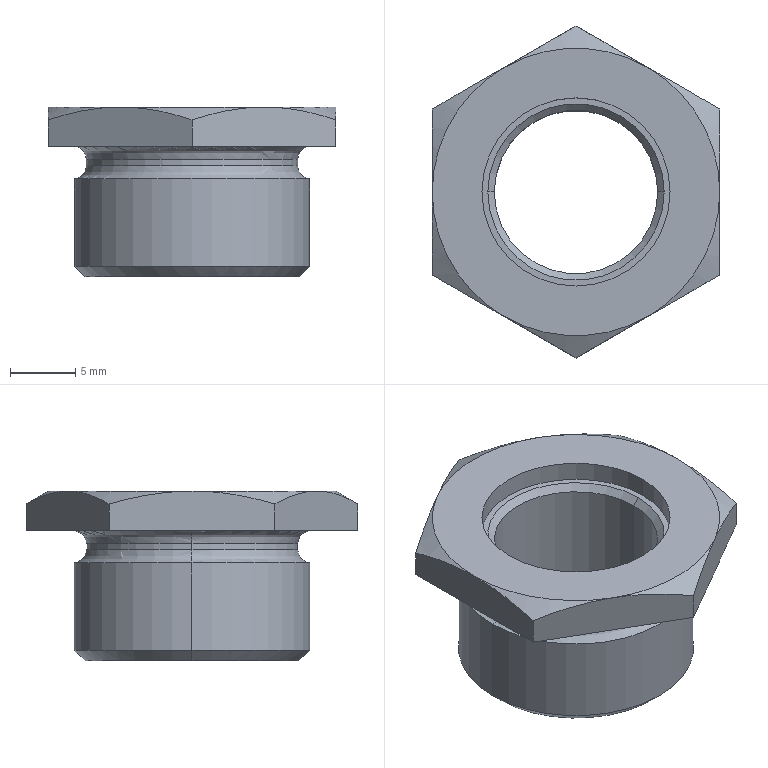Part | SolidWorks | features BaseBody 1 | 1 solid | 34 faces | box 22 x 25.403 x 13 mm | volume 2007 mm3 | cone 12 | plane 10 | cylinder 8 | torus 4 | commonest cylinder face diameters 12.5 x2 14.4 x2 16.2 x2 18 x2
STEP:
#1=CARTESIAN_POINT('',(49.25,110.5,49.));
#2=VERTEX_POINT('',#1);
#3=CARTESIAN_POINT('',(61.75,110.5,49.));
#4=VERTEX_POINT('',#3);
#5=CARTESIAN_POINT('',(55.5,110.5,49.));
#6=DIRECTION('',(0.,0.,1.));
#7=DIRECTION('',(1.,0.,0.));
#8=AXIS2_PLACEMENT_3D('',#5,#6,#7);
#9=CIRCLE('',#8,6.25);
#10=EDGE_CURVE('',#2,#4,#9,.T.);
#11=ORIENTED_EDGE('',*,*,#10,.F.);
#12=CARTESIAN_POINT('',(48.75,110.5,49.5));
#13=VERTEX_POINT('',#12);
#14=CARTESIAN_POINT('',(49.25,110.5,49.));
#15=DIRECTION('',(-0.7071,0.,0.7071));
#16=VECTOR('',#15,1000.);
#17=LINE('',#14,#16);
#18=EDGE_CURVE('',#2,#13,#17,.T.);
#19=ORIENTED_EDGE('',*,*,#18,.T.);
#20=CARTESIAN_POINT('',(62.25,110.5,49.5));
#21=VERTEX_POINT('',#20);
#22=CARTESIAN_POINT('',(55.5,110.5,49.5));
#23=DIRECTION('',(0.,0.,-1.));
#24=DIRECTION('',(1.,0.,0.));
#25=AXIS2_PLACEMENT_3D('',#22,#23,#24);
#26=CIRCLE('',#25,6.75);
#27=EDGE_CURVE('',#21,#13,#26,.T.);
#28=ORIENTED_EDGE('',*,*,#27,.F.);
#29=CARTESIAN_POINT('',(61.75,110.5,49.));
#30=DIRECTION('',(0.7071,0.,0.7071));
#31=VECTOR('',#30,1000.);
#32=LINE('',#29,#31);
#33=EDGE_CURVE('',#4,#21,#32,.T.);
#34=ORIENTED_EDGE('',*,*,#33,.F.);
#35=EDGE_LOOP('',(#11,#19,#28,#34));
#36=FACE_OUTER_BOUND('',#35,.T.);
#37=CARTESIAN_POINT('',(55.5,110.5,49.));
#38=DIRECTION('',(0.,0.,1.));
#39=DIRECTION('',(1.,0.,0.));
#40=AXIS2_PLACEMENT_3D('',#37,#38,#39);
#41=CONICAL_SURFACE('',#40,6.25,0.7854);
#42=ADVANCED_FACE('',(#36),#41,.F.);
#43=CARTESIAN_POINT('',(61.75,110.5,38.433));
#44=VERTEX_POINT('',#43);
#45=CARTESIAN_POINT('',(49.25,110.5,38.433));
#46=VERTEX_POINT('',#45);
#47=CARTESIAN_POINT('',(55.5,110.5,38.433));
#48=DIRECTION('',(0.,0.,-1.));
#49=DIRECTION('',(-1.,0.,0.));
#50=AXIS2_PLACEMENT_3D('',#47,#48,#49);
#51=CIRCLE('',#50,6.25);
#52=EDGE_CURVE('',#44,#46,#51,.T.);
#53=ORIENTED_EDGE('',*,*,#52,.F.);
#54=CARTESIAN_POINT('',(62.5,110.5,38.));
#55=VERTEX_POINT('',#54);
#56=CARTESIAN_POINT('',(62.5,110.5,38.));
#57=DIRECTION('',(0.866,0.,-0.5));
#58=VECTOR('',#57,1000.);
#59=LINE('',#56,#58);
#60=EDGE_CURVE('',#44,#55,#59,.T.);
#61=ORIENTED_EDGE('',*,*,#60,.T.);
#62=CARTESIAN_POINT('',(48.5,110.5,38.));
#63=VERTEX_POINT('',#62);
#64=CARTESIAN_POINT('',(55.5,110.5,38.));
#65=DIRECTION('',(0.,0.,-1.));
#66=DIRECTION('',(-1.,0.,0.));
#67=AXIS2_PLACEMENT_3D('',#64,#65,#66);
#68=CIRCLE('',#67,7.);
#69=EDGE_CURVE('',#55,#63,#68,.T.);
#70=ORIENTED_EDGE('',*,*,#69,.T.);
#71=CARTESIAN_POINT('',(48.5,110.5,38.));
#72=DIRECTION('',(-0.866,0.,-0.5));
#73=VECTOR('',#72,1000.);
#74=LINE('',#71,#73);
#75=EDGE_CURVE('',#46,#63,#74,.T.);
#76=ORIENTED_EDGE('',*,*,#75,.F.);
#77=EDGE_LOOP('',(#53,#61,#70,#76));
#78=FACE_OUTER_BOUND('',#77,.T.);
#79=CARTESIAN_POINT('',(55.5,110.5,38.));
#80=DIRECTION('',(0.,0.,-1.));
#81=DIRECTION('',(-1.,0.,0.));
#82=AXIS2_PLACEMENT_3D('',#79,#80,#81);
#83=CONICAL_SURFACE('',#82,7.,1.047);
#84=ADVANCED_FACE('',(#78),#83,.F.);
#85=ORIENTED_EDGE('',*,*,#10,.T.);
#86=CARTESIAN_POINT('',(61.75,110.5,38.));
#87=DIRECTION('',(0.,0.,-1.));
#88=VECTOR('',#87,1000.);
#89=LINE('',#86,#88);
#90=EDGE_CURVE('',#4,#44,#89,.T.);
#91=ORIENTED_EDGE('',*,*,#90,.T.);
#92=ORIENTED_EDGE('',*,*,#52,.T.);
#93=CARTESIAN_POINT('',(49.25,110.5,38.));
#94=DIRECTION('',(0.,0.,-1.));
#95=VECTOR('',#94,1000.);
#96=LINE('',#93,#95);
#97=EDGE_CURVE('',#2,#46,#96,.T.);
#98=ORIENTED_EDGE('',*,*,#97,.F.);
#99=EDGE_LOOP('',(#85,#91,#92,#98));
#100=FACE_OUTER_BOUND('',#99,.T.);
#101=CARTESIAN_POINT('',(55.5,110.5,38.));
#102=DIRECTION('',(0.,0.,-1.));
#103=DIRECTION('',(-1.,0.,0.));
#104=AXIS2_PLACEMENT_3D('',#101,#102,#103);
#105=CYLINDRICAL_SURFACE('',#104,6.25);
#106=ADVANCED_FACE('',(#100),#105,.F.);
#107=CARTESIAN_POINT('',(48.3,110.5,49.5));
#108=VERTEX_POINT('',#107);
#109=CARTESIAN_POINT('',(62.7,110.5,49.5));
#110=VERTEX_POINT('',#109);
#111=CARTESIAN_POINT('',(55.5,110.5,49.5));
#112=DIRECTION('',(0.,0.,1.));
#113=DIRECTION('',(1.,0.,0.));
#114=AXIS2_PLACEMENT_3D('',#111,#112,#113);
#115=CIRCLE('',#114,7.2);
#116=EDGE_CURVE('',#108,#110,#115,.T.);
#117=ORIENTED_EDGE('',*,*,#116,.F.);
#118=CARTESIAN_POINT('',(48.3,110.5,51.));
#119=VERTEX_POINT('',#118);
#120=CARTESIAN_POINT('',(48.3,110.5,49.5));
#121=DIRECTION('',(0.,0.,1.));
#122=VECTOR('',#121,1000.);
#123=LINE('',#120,#122);
#124=EDGE_CURVE('',#108,#119,#123,.T.);
#125=ORIENTED_EDGE('',*,*,#124,.T.);
#126=CARTESIAN_POINT('',(62.7,110.5,51.));
#127=VERTEX_POINT('',#126);
#128=CARTESIAN_POINT('',(55.5,110.5,51.));
#129=DIRECTION('',(0.,0.,1.));
#130=DIRECTION('',(1.,0.,0.));
#131=AXIS2_PLACEMENT_3D('',#128,#129,#130);
#132=CIRCLE('',#131,7.2);
#133=EDGE_CURVE('',#119,#127,#132,.T.);
#134=ORIENTED_EDGE('',*,*,#133,.T.);
#135=CARTESIAN_POINT('',(62.7,110.5,49.5));
#136=DIRECTION('',(0.,0.,1.));
#137=VECTOR('',#136,1000.);
#138=LINE('',#135,#137);
#139=EDGE_CURVE('',#110,#127,#138,.T.);
#140=ORIENTED_EDGE('',*,*,#139,.F.);
#141=EDGE_LOOP('',(#117,#125,#134,#140));
#142=FACE_OUTER_BOUND('',#141,.T.);
#143=CARTESIAN_POINT('',(55.5,110.5,49.5));
#144=DIRECTION('',(0.,0.,1.));
#145=DIRECTION('',(1.,0.,0.));
#146=AXIS2_PLACEMENT_3D('',#143,#144,#145);
#147=CYLINDRICAL_SURFACE('',#146,7.2);
#148=ADVANCED_FACE('',(#142),#147,.F.);
#149=CARTESIAN_POINT('',(63.6,110.5,47.005));
#150=VERTEX_POINT('',#149);
#151=CARTESIAN_POINT('',(47.4,110.5,47.005));
#152=VERTEX_POINT('',#151);
#153=CARTESIAN_POINT('',(55.5,110.5,47.005));
#154=DIRECTION('',(0.,0.,-1.));
#155=DIRECTION('',(-1.,0.,0.));
#156=AXIS2_PLACEMENT_3D('',#153,#154,#155);
#157=CIRCLE('',#156,8.1);
#158=EDGE_CURVE('',#150,#152,#157,.T.);
#159=ORIENTED_EDGE('',*,*,#158,.F.);
#160=CARTESIAN_POINT('',(64.5,110.5,48.));
#161=VERTEX_POINT('',#160);
#162=CARTESIAN_POINT('',(64.6,110.5,47.005));
#163=DIRECTION('',(0.,1.,0.));
#164=DIRECTION('',(-1.,0.,0.));
#165=AXIS2_PLACEMENT_3D('',#162,#163,#164);
#166=CIRCLE('',#165,1.);
#167=EDGE_CURVE('',#150,#161,#166,.T.);
#168=ORIENTED_EDGE('',*,*,#167,.T.);
#169=CARTESIAN_POINT('',(46.5,110.5,48.));
#170=VERTEX_POINT('',#169);
#171=CARTESIAN_POINT('',(55.5,110.5,48.));
#172=DIRECTION('',(0.,0.,1.));
#173=DIRECTION('',(1.,0.,0.));
#174=AXIS2_PLACEMENT_3D('',#171,#172,#173);
#175=CIRCLE('',#174,9.);
#176=EDGE_CURVE('',#170,#161,#175,.T.);
#177=ORIENTED_EDGE('',*,*,#176,.F.);
#178=CARTESIAN_POINT('',(46.4,110.5,47.005));
#179=DIRECTION('',(0.,-1.,0.));
#180=DIRECTION('',(1.,0.,0.));
#181=AXIS2_PLACEMENT_3D('',#178,#179,#180);
#182=CIRCLE('',#181,1.);
#183=EDGE_CURVE('',#152,#170,#182,.T.);
#184=ORIENTED_EDGE('',*,*,#183,.F.);
#185=EDGE_LOOP('',(#159,#168,#177,#184));
#186=FACE_OUTER_BOUND('',#185,.T.);
#187=CARTESIAN_POINT('',(55.5,110.5,47.005));
#188=DIRECTION('',(0.,0.,-1.));
#189=DIRECTION('',(-1.,0.,0.));
#190=AXIS2_PLACEMENT_3D('',#187,#188,#189);
#191=TOROIDAL_SURFACE('',#190,9.1,1.);
#192=ADVANCED_FACE('',(#186),#191,.F.);
#193=CARTESIAN_POINT('',(55.5,110.5,47.005));
#194=DIRECTION('',(0.,0.,-1.));
#195=DIRECTION('',(-1.,0.,0.));
#196=AXIS2_PLACEMENT_3D('',#193,#194,#195);
#197=CIRCLE('',#196,8.1);
#198=EDGE_CURVE('',#152,#150,#197,.T.);
#199=ORIENTED_EDGE('',*,*,#198,.T.);
#200=CARTESIAN_POINT('',(63.6,110.5,46.495));
#201=VERTEX_POINT('',#200);
#202=CARTESIAN_POINT('',(63.6,110.5,38.));
#203=DIRECTION('',(0.,0.,-1.));
#204=VECTOR('',#203,1000.);
#205=LINE('',#202,#204);
#206=EDGE_CURVE('',#150,#201,#205,.T.);
#207=ORIENTED_EDGE('',*,*,#206,.T.);
#208=CARTESIAN_POINT('',(47.4,110.5,46.495));
#209=VERTEX_POINT('',#208);
#210=CARTESIAN_POINT('',(55.5,110.5,46.495));
#211=DIRECTION('',(0.,0.,-1.));
#212=DIRECTION('',(-1.,0.,0.));
#213=AXIS2_PLACEMENT_3D('',#210,#211,#212);
#214=CIRCLE('',#213,8.1);
#215=EDGE_CURVE('',#209,#201,#214,.T.);
#216=ORIENTED_EDGE('',*,*,#215,.F.);
#217=CARTESIAN_POINT('',(47.4,110.5,38.));
#218=DIRECTION('',(0.,0.,-1.));
#219=VECTOR('',#218,1000.);
#220=LINE('',#217,#219);
#221=EDGE_CURVE('',#152,#209,#220,.T.);
#222=ORIENTED_EDGE('',*,*,#221,.F.);
#223=EDGE_LOOP('',(#199,#207,#216,#222));
#224=FACE_OUTER_BOUND('',#223,.T.);
#225=CARTESIAN_POINT('',(55.5,110.5,38.));
#226=DIRECTION('',(0.,0.,-1.));
#227=DIRECTION('',(-1.,0.,0.));
#228=AXIS2_PLACEMENT_3D('',#225,#226,#227);
#229=CYLINDRICAL_SURFACE('',#228,8.1);
#230=ADVANCED_FACE('',(#224),#229,.T.);
#231=CARTESIAN_POINT('',(64.5,110.5,45.5));
#232=VERTEX_POINT('',#231);
#233=CARTESIAN_POINT('',(46.5,110.5,45.5));
#234=VERTEX_POINT('',#233);
#235=CARTESIAN_POINT('',(55.5,110.5,45.5));
#236=DIRECTION('',(0.,0.,-1.));
#237=DIRECTION('',(-1.,0.,0.));
#238=AXIS2_PLACEMENT_3D('',#235,#236,#237);
#239=CIRCLE('',#238,9.);
#240=EDGE_CURVE('',#232,#234,#239,.T.);
#241=ORIENTED_EDGE('',*,*,#240,.F.);
#242=CARTESIAN_POINT('',(64.6,110.5,46.495));
#243=DIRECTION('',(0.,1.,0.));
#244=DIRECTION('',(-1.,0.,0.));
#245=AXIS2_PLACEMENT_3D('',#242,#243,#244);
#246=CIRCLE('',#245,1.);
#247=EDGE_CURVE('',#232,#201,#246,.T.);
#248=ORIENTED_EDGE('',*,*,#247,.T.);
#249=CARTESIAN_POINT('',(55.5,110.5,46.495));
#250=DIRECTION('',(0.,0.,-1.));
#251=DIRECTION('',(-1.,0.,0.));
#252=AXIS2_PLACEMENT_3D('',#249,#250,#251);
#253=CIRCLE('',#252,8.1);
#254=EDGE_CURVE('',#201,#209,#253,.T.);
#255=ORIENTED_EDGE('',*,*,#254,.T.);
#256=CARTESIAN_POINT('',(46.4,110.5,46.495));
#257=DIRECTION('',(0.,-1.,0.));
#258=DIRECTION('',(1.,0.,0.));
#259=AXIS2_PLACEMENT_3D('',#256,#257,#258);
#260=CIRCLE('',#259,1.);
#261=EDGE_CURVE('',#234,#209,#260,.T.);
#262=ORIENTED_EDGE('',*,*,#261,.F.);
#263=EDGE_LOOP('',(#241,#248,#255,#262));
#264=FACE_OUTER_BOUND('',#263,.T.);
#265=CARTESIAN_POINT('',(55.5,110.5,46.495));
#266=DIRECTION('',(0.,0.,-1.));
#267=DIRECTION('',(-1.,0.,0.));
#268=AXIS2_PLACEMENT_3D('',#265,#266,#267);
#269=TOROIDAL_SURFACE('',#268,9.1,1.);
#270=ADVANCED_FACE('',(#264),#269,.F.);
#271=CARTESIAN_POINT('',(55.5,110.5,45.5));
#272=DIRECTION('',(0.,0.,-1.));
#273=DIRECTION('',(-1.,0.,0.));
#274=AXIS2_PLACEMENT_3D('',#271,#272,#273);
#275=CIRCLE('',#274,9.);
#276=EDGE_CURVE('',#234,#232,#275,.T.);
#277=ORIENTED_EDGE('',*,*,#276,.T.);
#278=CARTESIAN_POINT('',(64.5,110.5,38.8));
#279=VERTEX_POINT('',#278);
#280=CARTESIAN_POINT('',(64.5,110.5,38.));
#281=DIRECTION('',(0.,0.,-1.));
#282=VECTOR('',#281,1000.);
#283=LINE('',#280,#282);
#284=EDGE_CURVE('',#232,#279,#283,.T.);
#285=ORIENTED_EDGE('',*,*,#284,.T.);
#286=CARTESIAN_POINT('',(46.5,110.5,38.8));
#287=VERTEX_POINT('',#286);
#288=CARTESIAN_POINT('',(55.5,110.5,38.8));
#289=DIRECTION('',(0.,0.,-1.));
#290=DIRECTION('',(-1.,0.,0.));
#291=AXIS2_PLACEMENT_3D('',#288,#289,#290);
#292=CIRCLE('',#291,9.);
#293=EDGE_CURVE('',#287,#279,#292,.T.);
#294=ORIENTED_EDGE('',*,*,#293,.F.);
#295=CARTESIAN_POINT('',(46.5,110.5,38.));
#296=DIRECTION('',(0.,0.,-1.));
#297=VECTOR('',#296,1000.);
#298=LINE('',#295,#297);
#299=EDGE_CURVE('',#234,#287,#298,.T.);
#300=ORIENTED_EDGE('',*,*,#299,.F.);
#301=EDGE_LOOP('',(#277,#285,#294,#300));
#302=FACE_OUTER_BOUND('',#301,.T.);
#303=CARTESIAN_POINT('',(55.5,110.5,38.));
#304=DIRECTION('',(0.,0.,-1.));
#305=DIRECTION('',(-1.,0.,0.));
#306=AXIS2_PLACEMENT_3D('',#303,#304,#305);
#307=CYLINDRICAL_SURFACE('',#306,9.);
#308=ADVANCED_FACE('',(#302),#307,.T.);
#309=CARTESIAN_POINT('',(47.3,110.5,38.));
#310=VERTEX_POINT('',#309);
#311=CARTESIAN_POINT('',(63.7,110.5,38.));
#312=VERTEX_POINT('',#311);
#313=CARTESIAN_POINT('',(55.5,110.5,38.));
#314=DIRECTION('',(0.,0.,-1.));
#315=DIRECTION('',(-1.,0.,0.));
#316=AXIS2_PLACEMENT_3D('',#313,#314,#315);
#317=CIRCLE('',#316,8.2);
#318=EDGE_CURVE('',#310,#312,#317,.T.);
#319=ORIENTED_EDGE('',*,*,#318,.F.);
#320=CARTESIAN_POINT('',(47.3,110.5,38.));
#321=DIRECTION('',(-0.7071,0.,0.7071));
#322=VECTOR('',#321,1000.);
#323=LINE('',#320,#322);
#324=EDGE_CURVE('',#310,#287,#323,.T.);
#325=ORIENTED_EDGE('',*,*,#324,.T.);
#326=ORIENTED_EDGE('',*,*,#293,.T.);
#327=CARTESIAN_POINT('',(63.7,110.5,38.));
#328=DIRECTION('',(0.7071,0.,0.7071));
#329=VECTOR('',#328,1000.);
#330=LINE('',#327,#329);
#331=EDGE_CURVE('',#312,#279,#330,.T.);
#332=ORIENTED_EDGE('',*,*,#331,.F.);
#333=EDGE_LOOP('',(#319,#325,#326,#332));
#334=FACE_OUTER_BOUND('',#333,.T.);
#335=CARTESIAN_POINT('',(55.5,110.5,38.));
#336=DIRECTION('',(0.,0.,1.));
#337=DIRECTION('',(1.,0.,0.));
#338=AXIS2_PLACEMENT_3D('',#335,#336,#337);
#339=CONICAL_SURFACE('',#338,8.2,0.7854);
#340=ADVANCED_FACE('',(#334),#339,.T.);
#341=CARTESIAN_POINT('',(44.5,104.149,50.018));
#342=VERTEX_POINT('',#341);
#343=CARTESIAN_POINT('',(50.,100.974,51.));
#344=VERTEX_POINT('',#343);
#345=CARTESIAN_POINT('',(44.5,104.149,50.018));
#346=CARTESIAN_POINT('',(45.4,103.63,50.317));
#347=CARTESIAN_POINT('',(46.306,103.106,50.565));
#348=CARTESIAN_POINT('',(48.138,102.049,50.906));
#349=CARTESIAN_POINT('',(49.063,101.515,51.));
#350=CARTESIAN_POINT('',(50.,100.974,51.));
#351=B_SPLINE_CURVE_WITH_KNOTS('',3,(#345,#346,#347,#348,#349,#350),.UNSPECIFIED.,.F.,.F.,(4,2,4),(0.000000238,0.003213,0.006426),.UNSPECIFIED.);
#352=EDGE_CURVE('',#342,#344,#351,.T.);
#353=ORIENTED_EDGE('',*,*,#352,.F.);
#354=CARTESIAN_POINT('',(44.5,104.149,48.));
#355=VERTEX_POINT('',#354);
#356=CARTESIAN_POINT('',(44.5,104.149,97.606));
#357=DIRECTION('',(0.,0.,-1.));
#358=VECTOR('',#357,1000.);
#359=LINE('',#356,#358);
#360=EDGE_CURVE('',#342,#355,#359,.T.);
#361=ORIENTED_EDGE('',*,*,#360,.T.);
#362=CARTESIAN_POINT('',(55.5,97.798,48.));
#363=VERTEX_POINT('',#362);
#364=CARTESIAN_POINT('',(44.5,104.149,48.));
#365=DIRECTION('',(0.866,-0.5,0.));
#366=VECTOR('',#365,1000.);
#367=LINE('',#364,#366);
#368=EDGE_CURVE('',#355,#363,#367,.T.);
#369=ORIENTED_EDGE('',*,*,#368,.T.);
#370=CARTESIAN_POINT('',(55.5,97.798,50.018));
#371=VERTEX_POINT('',#370);
#372=CARTESIAN_POINT('',(55.5,97.798,97.606));
#373=DIRECTION('',(0.,0.,-1.));
#374=VECTOR('',#373,1000.);
#375=LINE('',#372,#374);
#376=EDGE_CURVE('',#371,#363,#375,.T.);
#377=ORIENTED_EDGE('',*,*,#376,.F.);
#378=CARTESIAN_POINT('',(50.,100.974,51.));
#379=CARTESIAN_POINT('',(50.467,100.704,51.));
#380=CARTESIAN_POINT('',(50.936,100.434,50.977));
#381=CARTESIAN_POINT('',(51.863,99.898,50.887));
#382=CARTESIAN_POINT('',(52.324,99.632,50.82));
#383=CARTESIAN_POINT('',(53.698,98.839,50.564));
#384=CARTESIAN_POINT('',(54.603,98.316,50.317));
#385=CARTESIAN_POINT('',(55.5,97.798,50.018));
#386=B_SPLINE_CURVE_WITH_KNOTS('',3,(#378,#379,#380,#381,#382,#383,#384,#385),.UNSPECIFIED.,.F.,.F.,(4,2,2,4),(0.006426,0.008027,0.009627,0.01283),.UNSPECIFIED.);
#387=EDGE_CURVE('',#344,#371,#386,.T.);
#388=ORIENTED_EDGE('',*,*,#387,.F.);
#389=EDGE_LOOP('',(#353,#361,#369,#377,#388));
#390=FACE_OUTER_BOUND('',#389,.T.);
#391=CARTESIAN_POINT('',(44.5,104.149,97.606));
#392=DIRECTION('',(0.5,0.866,0.));
#393=DIRECTION('',(-0.866,0.5,0.));
#394=AXIS2_PLACEMENT_3D('',#391,#392,#393);
#395=PLANE('',#394);
#396=ADVANCED_FACE('',(#390),#395,.F.);
#397=CARTESIAN_POINT('',(44.5,116.851,50.018));
#398=VERTEX_POINT('',#397);
#399=CARTESIAN_POINT('',(44.5,110.5,51.));
#400=VERTEX_POINT('',#399);
#401=CARTESIAN_POINT('',(44.5,116.851,50.018));
#402=CARTESIAN_POINT('',(44.5,115.824,50.314));
#403=CARTESIAN_POINT('',(44.5,114.784,50.561));
#404=CARTESIAN_POINT('',(44.5,113.194,50.819));
#405=CARTESIAN_POINT('',(44.5,112.659,50.886));
#406=CARTESIAN_POINT('',(44.5,111.577,50.977));
#407=CARTESIAN_POINT('',(44.5,111.037,51.));
#408=CARTESIAN_POINT('',(44.5,110.5,51.));
#409=B_SPLINE_CURVE_WITH_KNOTS('',3,(#401,#402,#403,#404,#405,#406,#407,#408),.UNSPECIFIED.,.F.,.F.,(4,2,2,4),(0.02901,0.03222,0.03383,0.03544),.UNSPECIFIED.);
#410=EDGE_CURVE('',#398,#400,#409,.T.);
#411=ORIENTED_EDGE('',*,*,#410,.F.);
#412=CARTESIAN_POINT('',(44.5,116.851,48.));
#413=VERTEX_POINT('',#412);
#414=CARTESIAN_POINT('',(44.5,116.851,97.606));
#415=DIRECTION('',(0.,0.,-1.));
#416=VECTOR('',#415,1000.);
#417=LINE('',#414,#416);
#418=EDGE_CURVE('',#398,#413,#417,.T.);
#419=ORIENTED_EDGE('',*,*,#418,.T.);
#420=CARTESIAN_POINT('',(44.5,116.851,48.));
#421=DIRECTION('',(0.,-1.,0.));
#422=VECTOR('',#421,1000.);
#423=LINE('',#420,#422);
#424=EDGE_CURVE('',#413,#355,#423,.T.);
#425=ORIENTED_EDGE('',*,*,#424,.T.);
#426=ORIENTED_EDGE('',*,*,#360,.F.);
#427=CARTESIAN_POINT('',(44.5,110.5,51.));
#428=CARTESIAN_POINT('',(44.5,109.426,51.));
#429=CARTESIAN_POINT('',(44.5,108.36,50.908));
#430=CARTESIAN_POINT('',(44.5,106.24,50.566));
#431=CARTESIAN_POINT('',(44.5,105.183,50.316));
#432=CARTESIAN_POINT('',(44.5,104.149,50.018));
#433=B_SPLINE_CURVE_WITH_KNOTS('',3,(#427,#428,#429,#430,#431,#432),.UNSPECIFIED.,.F.,.F.,(4,2,4),(0.03544,0.03866,0.04187),.UNSPECIFIED.);
#434=EDGE_CURVE('',#400,#342,#433,.T.);
#435=ORIENTED_EDGE('',*,*,#434,.F.);
#436=EDGE_LOOP('',(#411,#419,#425,#426,#435));
#437=FACE_OUTER_BOUND('',#436,.T.);
#438=CARTESIAN_POINT('',(44.5,116.851,97.606));
#439=DIRECTION('',(1.,0.,0.));
#440=DIRECTION('',(0.,1.,0.));
#441=AXIS2_PLACEMENT_3D('',#438,#439,#440);
#442=PLANE('',#441);
#443=ADVANCED_FACE('',(#437),#442,.F.);
#444=CARTESIAN_POINT('',(55.5,123.202,50.018));
#445=VERTEX_POINT('',#444);
#446=CARTESIAN_POINT('',(50.,120.026,51.));
#447=VERTEX_POINT('',#446);
#448=CARTESIAN_POINT('',(55.5,123.202,50.018));
#449=CARTESIAN_POINT('',(54.6,122.682,50.317));
#450=CARTESIAN_POINT('',(53.694,122.159,50.565));
#451=CARTESIAN_POINT('',(51.862,121.102,50.906));
#452=CARTESIAN_POINT('',(50.937,120.567,51.));
#453=CARTESIAN_POINT('',(50.,120.026,51.));
#454=B_SPLINE_CURVE_WITH_KNOTS('',3,(#448,#449,#450,#451,#452,#453),.UNSPECIFIED.,.F.,.F.,(4,2,4),(0.000000238,0.003213,0.006426),.UNSPECIFIED.);
#455=EDGE_CURVE('',#445,#447,#454,.T.);
#456=ORIENTED_EDGE('',*,*,#455,.F.);
#457=CARTESIAN_POINT('',(55.5,123.202,48.));
#458=VERTEX_POINT('',#457);
#459=CARTESIAN_POINT('',(55.5,123.202,97.606));
#460=DIRECTION('',(0.,0.,-1.));
#461=VECTOR('',#460,1000.);
#462=LINE('',#459,#461);
#463=EDGE_CURVE('',#445,#458,#462,.T.);
#464=ORIENTED_EDGE('',*,*,#463,.T.);
#465=CARTESIAN_POINT('',(55.5,123.202,48.));
#466=DIRECTION('',(-0.866,-0.5,0.));
#467=VECTOR('',#466,1000.);
#468=LINE('',#465,#467);
#469=EDGE_CURVE('',#458,#413,#468,.T.);
#470=ORIENTED_EDGE('',*,*,#469,.T.);
#471=ORIENTED_EDGE('',*,*,#418,.F.);
#472=CARTESIAN_POINT('',(50.,120.026,51.));
#473=CARTESIAN_POINT('',(49.533,119.757,51.));
#474=CARTESIAN_POINT('',(49.064,119.486,50.977));
#475=CARTESIAN_POINT('',(48.137,118.951,50.887));
#476=CARTESIAN_POINT('',(47.676,118.685,50.82));
#477=CARTESIAN_POINT('',(46.302,117.891,50.564));
#478=CARTESIAN_POINT('',(45.397,117.369,50.317));
#479=CARTESIAN_POINT('',(44.5,116.851,50.018));
#480=B_SPLINE_CURVE_WITH_KNOTS('',3,(#472,#473,#474,#475,#476,#477,#478,#479),.UNSPECIFIED.,.F.,.F.,(4,2,2,4),(0.006426,0.008027,0.009627,0.01283),.UNSPECIFIED.);
#481=EDGE_CURVE('',#447,#398,#480,.T.);
#482=ORIENTED_EDGE('',*,*,#481,.F.);
#483=EDGE_LOOP('',(#456,#464,#470,#471,#482));
#484=FACE_OUTER_BOUND('',#483,.T.);
#485=CARTESIAN_POINT('',(55.5,123.202,97.606));
#486=DIRECTION('',(0.5,-0.866,0.));
#487=DIRECTION('',(0.866,0.5,0.));
#488=AXIS2_PLACEMENT_3D('',#485,#486,#487);
#489=PLANE('',#488);
#490=ADVANCED_FACE('',(#484),#489,.F.);
#491=CARTESIAN_POINT('',(66.5,116.851,50.018));
#492=VERTEX_POINT('',#491);
#493=CARTESIAN_POINT('',(61.,120.026,51.));
#494=VERTEX_POINT('',#493);
#495=CARTESIAN_POINT('',(66.5,116.851,50.018));
#496=CARTESIAN_POINT('',(65.6,117.37,50.317));
#497=CARTESIAN_POINT('',(64.694,117.894,50.565));
#498=CARTESIAN_POINT('',(62.862,118.951,50.906));
#499=CARTESIAN_POINT('',(61.937,119.485,51.));
#500=CARTESIAN_POINT('',(61.,120.026,51.));
#501=B_SPLINE_CURVE_WITH_KNOTS('',3,(#495,#496,#497,#498,#499,#500),.UNSPECIFIED.,.F.,.F.,(4,2,4),(0.000000238,0.003213,0.006426),.UNSPECIFIED.);
#502=EDGE_CURVE('',#492,#494,#501,.T.);
#503=ORIENTED_EDGE('',*,*,#502,.F.);
#504=CARTESIAN_POINT('',(66.5,116.851,48.));
#505=VERTEX_POINT('',#504);
#506=CARTESIAN_POINT('',(66.5,116.851,97.606));
#507=DIRECTION('',(0.,0.,-1.));
#508=VECTOR('',#507,1000.);
#509=LINE('',#506,#508);
#510=EDGE_CURVE('',#492,#505,#509,.T.);
#511=ORIENTED_EDGE('',*,*,#510,.T.);
#512=CARTESIAN_POINT('',(66.5,116.851,48.));
#513=DIRECTION('',(-0.866,0.5,0.));
#514=VECTOR('',#513,1000.);
#515=LINE('',#512,#514);
#516=EDGE_CURVE('',#505,#458,#515,.T.);
#517=ORIENTED_EDGE('',*,*,#516,.T.);
#518=ORIENTED_EDGE('',*,*,#463,.F.);
#519=CARTESIAN_POINT('',(61.,120.026,51.));
#520=CARTESIAN_POINT('',(60.533,120.296,51.));
#521=CARTESIAN_POINT('',(60.064,120.566,50.977));
#522=CARTESIAN_POINT('',(59.137,121.102,50.887));
#523=CARTESIAN_POINT('',(58.676,121.368,50.82));
#524=CARTESIAN_POINT('',(57.302,122.161,50.564));
#525=CARTESIAN_POINT('',(56.397,122.684,50.317));
#526=CARTESIAN_POINT('',(55.5,123.202,50.018));
#527=B_SPLINE_CURVE_WITH_KNOTS('',3,(#519,#520,#521,#522,#523,#524,#525,#526),.UNSPECIFIED.,.F.,.F.,(4,2,2,4),(0.006426,0.008027,0.009627,0.01283),.UNSPECIFIED.);
#528=EDGE_CURVE('',#494,#445,#527,.T.);
#529=ORIENTED_EDGE('',*,*,#528,.F.);
#530=EDGE_LOOP('',(#503,#511,#517,#518,#529));
#531=FACE_OUTER_BOUND('',#530,.T.);
#532=CARTESIAN_POINT('',(66.5,116.851,97.606));
#533=DIRECTION('',(-0.5,-0.866,0.));
#534=DIRECTION('',(0.866,-0.5,0.));
#535=AXIS2_PLACEMENT_3D('',#532,#533,#534);
#536=PLANE('',#535);
#537=ADVANCED_FACE('',(#531),#536,.F.);
#538=CARTESIAN_POINT('',(66.5,104.149,50.018));
#539=VERTEX_POINT('',#538);
#540=CARTESIAN_POINT('',(66.5,110.5,51.));
#541=VERTEX_POINT('',#540);
#542=CARTESIAN_POINT('',(66.5,104.149,50.018));
#543=CARTESIAN_POINT('',(66.5,105.183,50.316));
#544=CARTESIAN_POINT('',(66.5,106.24,50.566));
#545=CARTESIAN_POINT('',(66.5,108.36,50.908));
#546=CARTESIAN_POINT('',(66.5,109.426,51.));
#547=CARTESIAN_POINT('',(66.5,110.5,51.));
#548=B_SPLINE_CURVE_WITH_KNOTS('',3,(#542,#543,#544,#545,#546,#547),.UNSPECIFIED.,.F.,.F.,(4,2,4),(0.01164,0.01486,0.01807),.UNSPECIFIED.);
#549=EDGE_CURVE('',#539,#541,#548,.T.);
#550=ORIENTED_EDGE('',*,*,#549,.F.);
#551=CARTESIAN_POINT('',(66.5,104.149,48.));
#552=VERTEX_POINT('',#551);
#553=CARTESIAN_POINT('',(66.5,104.149,97.606));
#554=DIRECTION('',(0.,0.,-1.));
#555=VECTOR('',#554,1000.);
#556=LINE('',#553,#555);
#557=EDGE_CURVE('',#539,#552,#556,.T.);
#558=ORIENTED_EDGE('',*,*,#557,.T.);
#559=CARTESIAN_POINT('',(66.5,104.149,48.));
#560=DIRECTION('',(0.,1.,0.));
#561=VECTOR('',#560,1000.);
#562=LINE('',#559,#561);
#563=EDGE_CURVE('',#552,#505,#562,.T.);
#564=ORIENTED_EDGE('',*,*,#563,.T.);
#565=ORIENTED_EDGE('',*,*,#510,.F.);
#566=CARTESIAN_POINT('',(66.5,110.5,51.));
#567=CARTESIAN_POINT('',(66.5,111.037,51.));
#568=CARTESIAN_POINT('',(66.5,111.577,50.977));
#569=CARTESIAN_POINT('',(66.5,112.659,50.886));
#570=CARTESIAN_POINT('',(66.5,113.194,50.819));
#571=CARTESIAN_POINT('',(66.5,114.784,50.561));
#572=CARTESIAN_POINT('',(66.5,115.824,50.314));
#573=CARTESIAN_POINT('',(66.5,116.851,50.018));
#574=B_SPLINE_CURVE_WITH_KNOTS('',3,(#566,#567,#568,#569,#570,#571,#572,#573),.UNSPECIFIED.,.F.,.F.,(4,2,2,4),(0.01807,0.01968,0.02129,0.0245),.UNSPECIFIED.);
#575=EDGE_CURVE('',#541,#492,#574,.T.);
#576=ORIENTED_EDGE('',*,*,#575,.F.);
#577=EDGE_LOOP('',(#550,#558,#564,#565,#576));
#578=FACE_OUTER_BOUND('',#577,.T.);
#579=CARTESIAN_POINT('',(66.5,104.149,97.606));
#580=DIRECTION('',(-1.,0.,0.));
#581=DIRECTION('',(0.,-1.,0.));
#582=AXIS2_PLACEMENT_3D('',#579,#580,#581);
#583=PLANE('',#582);
#584=ADVANCED_FACE('',(#578),#583,.F.);
#585=CARTESIAN_POINT('',(61.,100.974,51.));
#586=VERTEX_POINT('',#585);
#587=CARTESIAN_POINT('',(55.5,97.798,50.018));
#588=CARTESIAN_POINT('',(56.4,98.318,50.317));
#589=CARTESIAN_POINT('',(57.306,98.841,50.565));
#590=CARTESIAN_POINT('',(59.138,99.898,50.906));
#591=CARTESIAN_POINT('',(60.063,100.433,51.));
#592=CARTESIAN_POINT('',(61.,100.974,51.));
#593=B_SPLINE_CURVE_WITH_KNOTS('',3,(#587,#588,#589,#590,#591,#592),.UNSPECIFIED.,.F.,.F.,(4,2,4),(0.000000238,0.003213,0.006426),.UNSPECIFIED.);
#594=EDGE_CURVE('',#371,#586,#593,.T.);
#595=ORIENTED_EDGE('',*,*,#594,.F.);
#596=ORIENTED_EDGE('',*,*,#376,.T.);
#597=CARTESIAN_POINT('',(55.5,97.798,48.));
#598=DIRECTION('',(0.866,0.5,0.));
#599=VECTOR('',#598,1000.);
#600=LINE('',#597,#599);
#601=EDGE_CURVE('',#363,#552,#600,.T.);
#602=ORIENTED_EDGE('',*,*,#601,.T.);
#603=ORIENTED_EDGE('',*,*,#557,.F.);
#604=CARTESIAN_POINT('',(61.,100.974,51.));
#605=CARTESIAN_POINT('',(61.467,101.243,51.));
#606=CARTESIAN_POINT('',(61.936,101.514,50.977));
#607=CARTESIAN_POINT('',(62.863,102.049,50.887));
#608=CARTESIAN_POINT('',(63.324,102.315,50.82));
#609=CARTESIAN_POINT('',(64.698,103.109,50.564));
#610=CARTESIAN_POINT('',(65.603,103.631,50.317));
#611=CARTESIAN_POINT('',(66.5,104.149,50.018));
#612=B_SPLINE_CURVE_WITH_KNOTS('',3,(#604,#605,#606,#607,#608,#609,#610,#611),.UNSPECIFIED.,.F.,.F.,(4,2,2,4),(0.006426,0.008027,0.009627,0.01283),.UNSPECIFIED.);
#613=EDGE_CURVE('',#586,#539,#612,.T.);
#614=ORIENTED_EDGE('',*,*,#613,.F.);
#615=EDGE_LOOP('',(#595,#596,#602,#603,#614));
#616=FACE_OUTER_BOUND('',#615,.T.);
#617=CARTESIAN_POINT('',(55.5,97.798,97.606));
#618=DIRECTION('',(-0.5,0.866,0.));
#619=DIRECTION('',(-0.866,-0.5,0.));
#620=AXIS2_PLACEMENT_3D('',#617,#618,#619);
#621=PLANE('',#620);
#622=ADVANCED_FACE('',(#616),#621,.F.);
#623=CARTESIAN_POINT('',(55.5,110.5,38.));
#624=DIRECTION('',(0.,0.,-1.));
#625=DIRECTION('',(-1.,0.,0.));
#626=AXIS2_PLACEMENT_3D('',#623,#624,#625);
#627=CIRCLE('',#626,7.);
#628=EDGE_CURVE('',#63,#55,#627,.T.);
#629=ORIENTED_EDGE('',*,*,#628,.F.);
#630=ORIENTED_EDGE('',*,*,#69,.F.);
#631=EDGE_LOOP('',(#629,#630));
#632=FACE_BOUND('',#631,.T.);
#633=CARTESIAN_POINT('',(55.5,110.5,38.));
#634=DIRECTION('',(0.,0.,-1.));
#635=DIRECTION('',(-1.,0.,0.));
#636=AXIS2_PLACEMENT_3D('',#633,#634,#635);
#637=CIRCLE('',#636,8.2);
#638=EDGE_CURVE('',#312,#310,#637,.T.);
#639=ORIENTED_EDGE('',*,*,#638,.T.);
#640=ORIENTED_EDGE('',*,*,#318,.T.);
#641=EDGE_LOOP('',(#639,#640));
#642=FACE_OUTER_BOUND('',#641,.T.);
#643=CARTESIAN_POINT('',(55.5,110.5,38.));
#644=DIRECTION('',(0.,0.,-1.));
#645=DIRECTION('',(-1.,0.,0.));
#646=AXIS2_PLACEMENT_3D('',#643,#644,#645);
#647=PLANE('',#646);
#648=ADVANCED_FACE('',(#632,#642),#647,.T.);
#649=ORIENTED_EDGE('',*,*,#324,.F.);
#650=ORIENTED_EDGE('',*,*,#638,.F.);
#651=ORIENTED_EDGE('',*,*,#331,.T.);
#652=CARTESIAN_POINT('',(55.5,110.5,38.8));
#653=DIRECTION('',(0.,0.,-1.));
#654=DIRECTION('',(-1.,0.,0.));
#655=AXIS2_PLACEMENT_3D('',#652,#653,#654);
#656=CIRCLE('',#655,9.);
#657=EDGE_CURVE('',#279,#287,#656,.T.);
#658=ORIENTED_EDGE('',*,*,#657,.T.);
#659=EDGE_LOOP('',(#649,#650,#651,#658));
#660=FACE_OUTER_BOUND('',#659,.T.);
#661=CARTESIAN_POINT('',(55.5,110.5,38.));
#662=DIRECTION('',(0.,0.,1.));
#663=DIRECTION('',(1.,0.,0.));
#664=AXIS2_PLACEMENT_3D('',#661,#662,#663);
#665=CONICAL_SURFACE('',#664,8.2,0.7854);
#666=ADVANCED_FACE('',(#660),#665,.T.);
#667=ORIENTED_EDGE('',*,*,#284,.F.);
#668=ORIENTED_EDGE('',*,*,#240,.T.);
#669=ORIENTED_EDGE('',*,*,#299,.T.);
#670=ORIENTED_EDGE('',*,*,#657,.F.);
#671=EDGE_LOOP('',(#667,#668,#669,#670));
#672=FACE_OUTER_BOUND('',#671,.T.);
#673=CARTESIAN_POINT('',(55.5,110.5,38.));
#674=DIRECTION('',(0.,0.,-1.));
#675=DIRECTION('',(-1.,0.,0.));
#676=AXIS2_PLACEMENT_3D('',#673,#674,#675);
#677=CYLINDRICAL_SURFACE('',#676,9.);
#678=ADVANCED_FACE('',(#672),#677,.T.);
#679=ORIENTED_EDGE('',*,*,#247,.F.);
#680=ORIENTED_EDGE('',*,*,#276,.F.);
#681=ORIENTED_EDGE('',*,*,#261,.T.);
#682=ORIENTED_EDGE('',*,*,#215,.T.);
#683=EDGE_LOOP('',(#679,#680,#681,#682));
#684=FACE_OUTER_BOUND('',#683,.T.);
#685=CARTESIAN_POINT('',(55.5,110.5,46.495));
#686=DIRECTION('',(0.,0.,-1.));
#687=DIRECTION('',(-1.,0.,0.));
#688=AXIS2_PLACEMENT_3D('',#685,#686,#687);
#689=TOROIDAL_SURFACE('',#688,9.1,1.);
#690=ADVANCED_FACE('',(#684),#689,.F.);
#691=ORIENTED_EDGE('',*,*,#206,.F.);
#692=ORIENTED_EDGE('',*,*,#158,.T.);
#693=ORIENTED_EDGE('',*,*,#221,.T.);
#694=ORIENTED_EDGE('',*,*,#254,.F.);
#695=EDGE_LOOP('',(#691,#692,#693,#694));
#696=FACE_OUTER_BOUND('',#695,.T.);
#697=CARTESIAN_POINT('',(55.5,110.5,38.));
#698=DIRECTION('',(0.,0.,-1.));
#699=DIRECTION('',(-1.,0.,0.));
#700=AXIS2_PLACEMENT_3D('',#697,#698,#699);
#701=CYLINDRICAL_SURFACE('',#700,8.1);
#702=ADVANCED_FACE('',(#696),#701,.T.);
#703=ORIENTED_EDGE('',*,*,#167,.F.);
#704=ORIENTED_EDGE('',*,*,#198,.F.);
#705=ORIENTED_EDGE('',*,*,#183,.T.);
#706=CARTESIAN_POINT('',(55.5,110.5,48.));
#707=DIRECTION('',(0.,0.,1.));
#708=DIRECTION('',(1.,0.,0.));
#709=AXIS2_PLACEMENT_3D('',#706,#707,#708);
#710=CIRCLE('',#709,9.);
#711=EDGE_CURVE('',#161,#170,#710,.T.);
#712=ORIENTED_EDGE('',*,*,#711,.F.);
#713=EDGE_LOOP('',(#703,#704,#705,#712));
#714=FACE_OUTER_BOUND('',#713,.T.);
#715=CARTESIAN_POINT('',(55.5,110.5,47.005));
#716=DIRECTION('',(0.,0.,-1.));
#717=DIRECTION('',(-1.,0.,0.));
#718=AXIS2_PLACEMENT_3D('',#715,#716,#717);
#719=TOROIDAL_SURFACE('',#718,9.1,1.);
#720=ADVANCED_FACE('',(#714),#719,.F.);
#721=ORIENTED_EDGE('',*,*,#176,.T.);
#722=ORIENTED_EDGE('',*,*,#711,.T.);
#723=EDGE_LOOP('',(#721,#722));
#724=FACE_BOUND('',#723,.T.);
#725=ORIENTED_EDGE('',*,*,#601,.F.);
#726=ORIENTED_EDGE('',*,*,#368,.F.);
#727=ORIENTED_EDGE('',*,*,#424,.F.);
#728=ORIENTED_EDGE('',*,*,#469,.F.);
#729=ORIENTED_EDGE('',*,*,#516,.F.);
#730=ORIENTED_EDGE('',*,*,#563,.F.);
#731=EDGE_LOOP('',(#725,#726,#727,#728,#729,#730));
#732=FACE_OUTER_BOUND('',#731,.T.);
#733=CARTESIAN_POINT('',(55.5,97.798,48.));
#734=DIRECTION('',(0.,0.,-1.));
#735=DIRECTION('',(-1.,0.,0.));
#736=AXIS2_PLACEMENT_3D('',#733,#734,#735);
#737=PLANE('',#736);
#738=ADVANCED_FACE('',(#724,#732),#737,.T.);
#739=ORIENTED_EDGE('',*,*,#434,.T.);
#740=ORIENTED_EDGE('',*,*,#352,.T.);
#741=CARTESIAN_POINT('',(55.5,110.5,51.));
#742=DIRECTION('',(0.,0.,-1.));
#743=DIRECTION('',(-1.,0.,0.));
#744=AXIS2_PLACEMENT_3D('',#741,#742,#743);
#745=CIRCLE('',#744,11.);
#746=EDGE_CURVE('',#344,#400,#745,.T.);
#747=ORIENTED_EDGE('',*,*,#746,.T.);
#748=EDGE_LOOP('',(#739,#740,#747));
#749=FACE_OUTER_BOUND('',#748,.T.);
#750=CARTESIAN_POINT('',(55.5,110.5,51.));
#751=DIRECTION('',(0.,0.,-1.));
#752=DIRECTION('',(1.,0.,0.));
#753=AXIS2_PLACEMENT_3D('',#750,#751,#752);
#754=CONICAL_SURFACE('',#753,11.,1.047);
#755=ADVANCED_FACE('',(#749),#754,.T.);
#756=ORIENTED_EDGE('',*,*,#387,.T.);
#757=ORIENTED_EDGE('',*,*,#594,.T.);
#758=CARTESIAN_POINT('',(55.5,110.5,51.));
#759=DIRECTION('',(0.,0.,-1.));
#760=DIRECTION('',(-1.,0.,0.));
#761=AXIS2_PLACEMENT_3D('',#758,#759,#760);
#762=CIRCLE('',#761,11.);
#763=EDGE_CURVE('',#586,#344,#762,.T.);
#764=ORIENTED_EDGE('',*,*,#763,.T.);
#765=EDGE_LOOP('',(#756,#757,#764));
#766=FACE_OUTER_BOUND('',#765,.T.);
#767=CARTESIAN_POINT('',(55.5,110.5,51.));
#768=DIRECTION('',(0.,0.,-1.));
#769=DIRECTION('',(1.,0.,0.));
#770=AXIS2_PLACEMENT_3D('',#767,#768,#769);
#771=CONICAL_SURFACE('',#770,11.,1.047);
#772=ADVANCED_FACE('',(#766),#771,.T.);
#773=ORIENTED_EDGE('',*,*,#549,.T.);
#774=CARTESIAN_POINT('',(55.5,110.5,51.));
#775=DIRECTION('',(0.,0.,-1.));
#776=DIRECTION('',(-1.,0.,0.));
#777=AXIS2_PLACEMENT_3D('',#774,#775,#776);
#778=CIRCLE('',#777,11.);
#779=EDGE_CURVE('',#541,#586,#778,.T.);
#780=ORIENTED_EDGE('',*,*,#779,.T.);
#781=ORIENTED_EDGE('',*,*,#613,.T.);
#782=EDGE_LOOP('',(#773,#780,#781));
#783=FACE_OUTER_BOUND('',#782,.T.);
#784=CARTESIAN_POINT('',(55.5,110.5,51.));
#785=DIRECTION('',(0.,0.,-1.));
#786=DIRECTION('',(1.,0.,0.));
#787=AXIS2_PLACEMENT_3D('',#784,#785,#786);
#788=CONICAL_SURFACE('',#787,11.,1.047);
#789=ADVANCED_FACE('',(#783),#788,.T.);
#790=ORIENTED_EDGE('',*,*,#502,.T.);
#791=CARTESIAN_POINT('',(55.5,110.5,51.));
#792=DIRECTION('',(0.,0.,1.));
#793=DIRECTION('',(1.,0.,0.));
#794=AXIS2_PLACEMENT_3D('',#791,#792,#793);
#795=CIRCLE('',#794,11.);
#796=EDGE_CURVE('',#541,#494,#795,.T.);
#797=ORIENTED_EDGE('',*,*,#796,.F.);
#798=ORIENTED_EDGE('',*,*,#575,.T.);
#799=EDGE_LOOP('',(#790,#797,#798));
#800=FACE_OUTER_BOUND('',#799,.T.);
#801=CARTESIAN_POINT('',(55.5,110.5,51.));
#802=DIRECTION('',(0.,0.,-1.));
#803=DIRECTION('',(1.,0.,0.));
#804=AXIS2_PLACEMENT_3D('',#801,#802,#803);
#805=CONICAL_SURFACE('',#804,11.,1.047);
#806=ADVANCED_FACE('',(#800),#805,.T.);
#807=ORIENTED_EDGE('',*,*,#455,.T.);
#808=CARTESIAN_POINT('',(55.5,110.5,51.));
#809=DIRECTION('',(0.,0.,-1.));
#810=DIRECTION('',(-1.,0.,0.));
#811=AXIS2_PLACEMENT_3D('',#808,#809,#810);
#812=CIRCLE('',#811,11.);
#813=EDGE_CURVE('',#447,#494,#812,.T.);
#814=ORIENTED_EDGE('',*,*,#813,.T.);
#815=ORIENTED_EDGE('',*,*,#528,.T.);
#816=EDGE_LOOP('',(#807,#814,#815));
#817=FACE_OUTER_BOUND('',#816,.T.);
#818=CARTESIAN_POINT('',(55.5,110.5,51.));
#819=DIRECTION('',(0.,0.,-1.));
#820=DIRECTION('',(1.,0.,0.));
#821=AXIS2_PLACEMENT_3D('',#818,#819,#820);
#822=CONICAL_SURFACE('',#821,11.,1.047);
#823=ADVANCED_FACE('',(#817),#822,.T.);
#824=ORIENTED_EDGE('',*,*,#481,.T.);
#825=ORIENTED_EDGE('',*,*,#410,.T.);
#826=CARTESIAN_POINT('',(55.5,110.5,51.));
#827=DIRECTION('',(0.,0.,-1.));
#828=DIRECTION('',(-1.,0.,0.));
#829=AXIS2_PLACEMENT_3D('',#826,#827,#828);
#830=CIRCLE('',#829,11.);
#831=EDGE_CURVE('',#400,#447,#830,.T.);
#832=ORIENTED_EDGE('',*,*,#831,.T.);
#833=EDGE_LOOP('',(#824,#825,#832));
#834=FACE_OUTER_BOUND('',#833,.T.);
#835=CARTESIAN_POINT('',(55.5,110.5,51.));
#836=DIRECTION('',(0.,0.,-1.));
#837=DIRECTION('',(1.,0.,0.));
#838=AXIS2_PLACEMENT_3D('',#835,#836,#837);
#839=CONICAL_SURFACE('',#838,11.,1.047);
#840=ADVANCED_FACE('',(#834),#839,.T.);
#841=CARTESIAN_POINT('',(55.5,110.5,51.));
#842=DIRECTION('',(0.,0.,1.));
#843=DIRECTION('',(1.,0.,0.));
#844=AXIS2_PLACEMENT_3D('',#841,#842,#843);
#845=CIRCLE('',#844,7.2);
#846=EDGE_CURVE('',#127,#119,#845,.T.);
#847=ORIENTED_EDGE('',*,*,#846,.F.);
#848=ORIENTED_EDGE('',*,*,#133,.F.);
#849=EDGE_LOOP('',(#847,#848));
#850=FACE_BOUND('',#849,.T.);
#851=ORIENTED_EDGE('',*,*,#831,.F.);
#852=ORIENTED_EDGE('',*,*,#746,.F.);
#853=ORIENTED_EDGE('',*,*,#763,.F.);
#854=ORIENTED_EDGE('',*,*,#779,.F.);
#855=ORIENTED_EDGE('',*,*,#796,.T.);
#856=ORIENTED_EDGE('',*,*,#813,.F.);
#857=EDGE_LOOP('',(#851,#852,#853,#854,#855,#856));
#858=FACE_OUTER_BOUND('',#857,.T.);
#859=CARTESIAN_POINT('',(55.5,110.5,51.));
#860=DIRECTION('',(0.,0.,-1.));
#861=DIRECTION('',(-1.,0.,0.));
#862=AXIS2_PLACEMENT_3D('',#859,#860,#861);
#863=PLANE('',#862);
#864=ADVANCED_FACE('',(#850,#858),#863,.F.);
#865=ORIENTED_EDGE('',*,*,#124,.F.);
#866=CARTESIAN_POINT('',(55.5,110.5,49.5));
#867=DIRECTION('',(0.,0.,1.));
#868=DIRECTION('',(1.,0.,0.));
#869=AXIS2_PLACEMENT_3D('',#866,#867,#868);
#870=CIRCLE('',#869,7.2);
#871=EDGE_CURVE('',#110,#108,#870,.T.);
#872=ORIENTED_EDGE('',*,*,#871,.F.);
#873=ORIENTED_EDGE('',*,*,#139,.T.);
#874=ORIENTED_EDGE('',*,*,#846,.T.);
#875=EDGE_LOOP('',(#865,#872,#873,#874));
#876=FACE_OUTER_BOUND('',#875,.T.);
#877=CARTESIAN_POINT('',(55.5,110.5,49.5));
#878=DIRECTION('',(0.,0.,1.));
#879=DIRECTION('',(1.,0.,0.));
#880=AXIS2_PLACEMENT_3D('',#877,#878,#879);
#881=CYLINDRICAL_SURFACE('',#880,7.2);
#882=ADVANCED_FACE('',(#876),#881,.F.);
#883=ORIENTED_EDGE('',*,*,#27,.T.);
#884=CARTESIAN_POINT('',(55.5,110.5,49.5));
#885=DIRECTION('',(0.,0.,-1.));
#886=DIRECTION('',(1.,0.,0.));
#887=AXIS2_PLACEMENT_3D('',#884,#885,#886);
#888=CIRCLE('',#887,6.75);
#889=EDGE_CURVE('',#13,#21,#888,.T.);
#890=ORIENTED_EDGE('',*,*,#889,.T.);
#891=EDGE_LOOP('',(#883,#890));
#892=FACE_BOUND('',#891,.T.);
#893=ORIENTED_EDGE('',*,*,#871,.T.);
#894=ORIENTED_EDGE('',*,*,#116,.T.);
#895=EDGE_LOOP('',(#893,#894));
#896=FACE_OUTER_BOUND('',#895,.T.);
#897=CARTESIAN_POINT('',(55.5,110.5,49.5));
#898=DIRECTION('',(0.,0.,1.));
#899=DIRECTION('',(1.,0.,0.));
#900=AXIS2_PLACEMENT_3D('',#897,#898,#899);
#901=PLANE('',#900);
#902=ADVANCED_FACE('',(#892,#896),#901,.T.);
#903=ORIENTED_EDGE('',*,*,#90,.F.);
#904=CARTESIAN_POINT('',(55.5,110.5,49.));
#905=DIRECTION('',(0.,0.,1.));
#906=DIRECTION('',(1.,0.,0.));
#907=AXIS2_PLACEMENT_3D('',#904,#905,#906);
#908=CIRCLE('',#907,6.25);
#909=EDGE_CURVE('',#4,#2,#908,.T.);
#910=ORIENTED_EDGE('',*,*,#909,.T.);
#911=ORIENTED_EDGE('',*,*,#97,.T.);
#912=CARTESIAN_POINT('',(55.5,110.5,38.433));
#913=DIRECTION('',(0.,0.,-1.));
#914=DIRECTION('',(-1.,0.,0.));
#915=AXIS2_PLACEMENT_3D('',#912,#913,#914);
#916=CIRCLE('',#915,6.25);
#917=EDGE_CURVE('',#46,#44,#916,.T.);
#918=ORIENTED_EDGE('',*,*,#917,.T.);
#919=EDGE_LOOP('',(#903,#910,#911,#918));
#920=FACE_OUTER_BOUND('',#919,.T.);
#921=CARTESIAN_POINT('',(55.5,110.5,38.));
#922=DIRECTION('',(0.,0.,-1.));
#923=DIRECTION('',(-1.,0.,0.));
#924=AXIS2_PLACEMENT_3D('',#921,#922,#923);
#925=CYLINDRICAL_SURFACE('',#924,6.25);
#926=ADVANCED_FACE('',(#920),#925,.F.);
#927=ORIENTED_EDGE('',*,*,#60,.F.);
#928=ORIENTED_EDGE('',*,*,#917,.F.);
#929=ORIENTED_EDGE('',*,*,#75,.T.);
#930=ORIENTED_EDGE('',*,*,#628,.T.);
#931=EDGE_LOOP('',(#927,#928,#929,#930));
#932=FACE_OUTER_BOUND('',#931,.T.);
#933=CARTESIAN_POINT('',(55.5,110.5,38.));
#934=DIRECTION('',(0.,0.,-1.));
#935=DIRECTION('',(-1.,0.,0.));
#936=AXIS2_PLACEMENT_3D('',#933,#934,#935);
#937=CONICAL_SURFACE('',#936,7.,1.047);
#938=ADVANCED_FACE('',(#932),#937,.F.);
#939=ORIENTED_EDGE('',*,*,#18,.F.);
#940=ORIENTED_EDGE('',*,*,#909,.F.);
#941=ORIENTED_EDGE('',*,*,#33,.T.);
#942=ORIENTED_EDGE('',*,*,#889,.F.);
#943=EDGE_LOOP('',(#939,#940,#941,#942));
#944=FACE_OUTER_BOUND('',#943,.T.);
#945=CARTESIAN_POINT('',(55.5,110.5,49.));
#946=DIRECTION('',(0.,0.,1.));
#947=DIRECTION('',(1.,0.,0.));
#948=AXIS2_PLACEMENT_3D('',#945,#946,#947);
#949=CONICAL_SURFACE('',#948,6.25,0.7854);
#950=ADVANCED_FACE('',(#944),#949,.F.);
#951=CLOSED_SHELL('',(#42,#84,#106,#148,#192,#230,#270,#308,#340,#396,#443,#490,#537,#584,#622,#648,#666,#678,#690,#702,#720,#738,#755,#772,#789,#806,#823,#840,#864,#882,#902,#926,#938,#950));
#952=MANIFOLD_SOLID_BREP('',#951);
#953=CARTESIAN_POINT('',(0.,0.,0.));
#954=DIRECTION('',(0.,0.,1.));
#955=DIRECTION('',(1.,0.,0.));
#956=AXIS2_PLACEMENT_3D('',#953,#954,#955);
#957=(LENGTH_UNIT()NAMED_UNIT(*)SI_UNIT(.MILLI.,.METRE.));
#958=UNCERTAINTY_MEASURE_WITH_UNIT(LENGTH_MEASURE(0.00001),#957,'','');
#959=(NAMED_UNIT(*)PLANE_ANGLE_UNIT()SI_UNIT($,.RADIAN.));
#960=(NAMED_UNIT(*)SI_UNIT($,.STERADIAN.)SOLID_ANGLE_UNIT());
#961=(GEOMETRIC_REPRESENTATION_CONTEXT(3)GLOBAL_UNCERTAINTY_ASSIGNED_CONTEXT((#958))GLOBAL_UNIT_ASSIGNED_CONTEXT((#957,#959,#960))REPRESENTATION_CONTEXT('',''));
#962=ADVANCED_BREP_SHAPE_REPRESENTATION('',(#952,#956),#961);